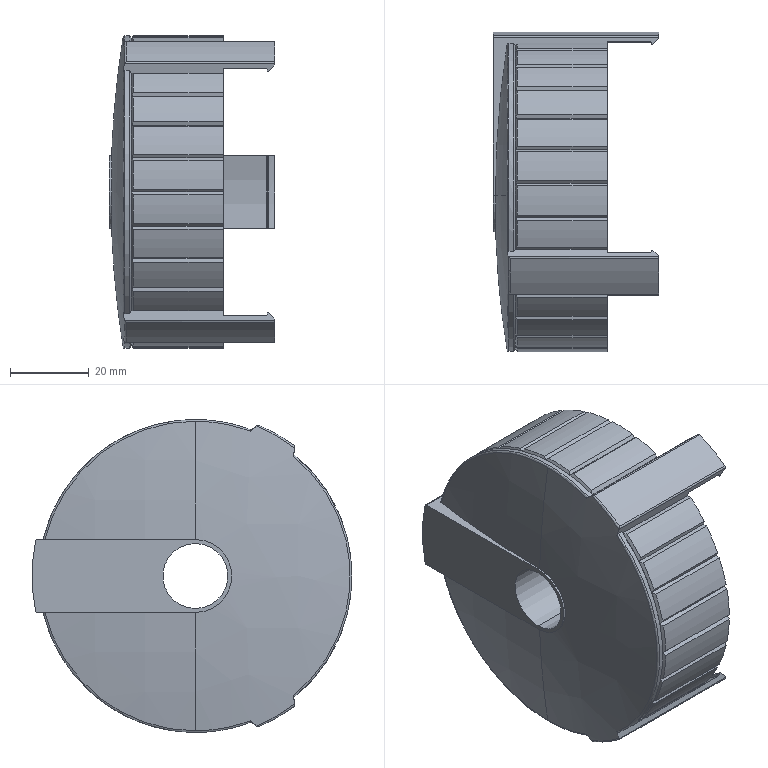Part | STEP file | PN_0032 | 1 solid | 199 faces | box 41.9 x 81.2 x 79.4 mm | volume 19535 mm3 | plane 73 | cylinder 72 | cone 35 | spline 19 | commonest cylinder face diameters 79.4 x29 1 x14 2 x7 0.5 x4 77.4 x4 75 x3